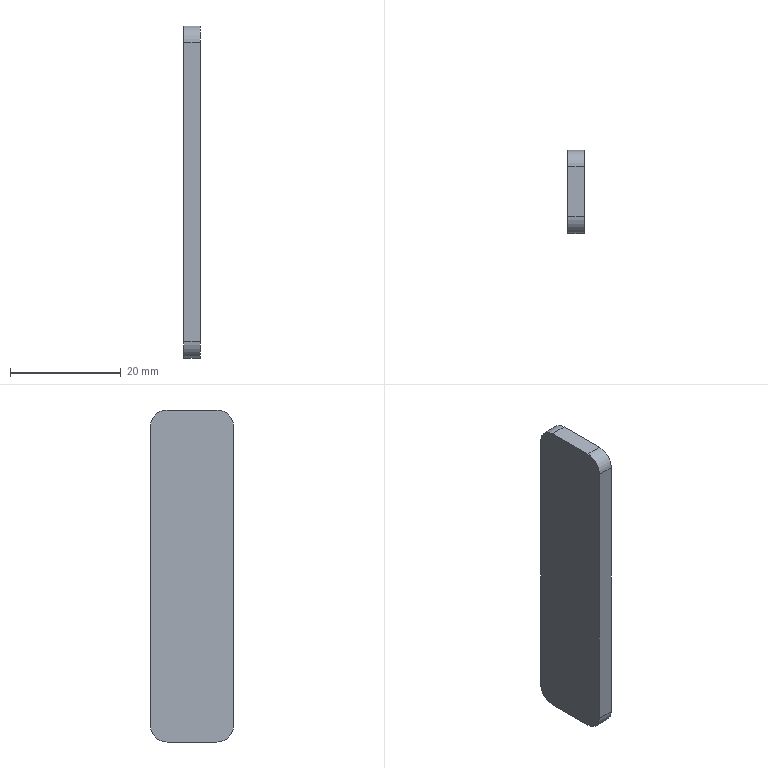Part | SolidWorks | features BaseBody 1 | 1 solid | 10 faces | box 3 x 15 x 60 mm | volume 2677 mm3 | plane 6 | cylinder 4 | commonest cylinder face diameters 6 x4
STEP:
#1=CARTESIAN_POINT('',(72.,-22.5,27.));
#2=VERTEX_POINT('',#1);
#3=CARTESIAN_POINT('',(72.,-25.5,30.));
#4=VERTEX_POINT('',#3);
#5=CARTESIAN_POINT('',(72.,-25.5,27.));
#6=DIRECTION('',(1.,0.,0.));
#7=DIRECTION('',(0.,1.,0.));
#8=AXIS2_PLACEMENT_3D('',#5,#6,#7);
#9=CIRCLE('',#8,3.);
#10=EDGE_CURVE('',#2,#4,#9,.T.);
#11=ORIENTED_EDGE('',*,*,#10,.F.);
#12=CARTESIAN_POINT('',(72.,-22.5,-27.));
#13=VERTEX_POINT('',#12);
#14=CARTESIAN_POINT('',(72.,-22.5,-27.));
#15=DIRECTION('',(0.,0.,1.));
#16=VECTOR('',#15,1000.);
#17=LINE('',#14,#16);
#18=EDGE_CURVE('',#13,#2,#17,.T.);
#19=ORIENTED_EDGE('',*,*,#18,.F.);
#20=CARTESIAN_POINT('',(72.,-25.5,-30.));
#21=VERTEX_POINT('',#20);
#22=CARTESIAN_POINT('',(72.,-25.5,-27.));
#23=DIRECTION('',(1.,0.,0.));
#24=DIRECTION('',(0.,0.,-1.));
#25=AXIS2_PLACEMENT_3D('',#22,#23,#24);
#26=CIRCLE('',#25,3.);
#27=EDGE_CURVE('',#21,#13,#26,.T.);
#28=ORIENTED_EDGE('',*,*,#27,.F.);
#29=CARTESIAN_POINT('',(72.,-34.5,-30.));
#30=VERTEX_POINT('',#29);
#31=CARTESIAN_POINT('',(72.,-34.5,-30.));
#32=DIRECTION('',(0.,1.,0.));
#33=VECTOR('',#32,1000.);
#34=LINE('',#31,#33);
#35=EDGE_CURVE('',#30,#21,#34,.T.);
#36=ORIENTED_EDGE('',*,*,#35,.F.);
#37=CARTESIAN_POINT('',(72.,-37.5,-27.));
#38=VERTEX_POINT('',#37);
#39=CARTESIAN_POINT('',(72.,-34.5,-27.));
#40=DIRECTION('',(1.,0.,0.));
#41=DIRECTION('',(0.,-1.,0.));
#42=AXIS2_PLACEMENT_3D('',#39,#40,#41);
#43=CIRCLE('',#42,3.);
#44=EDGE_CURVE('',#38,#30,#43,.T.);
#45=ORIENTED_EDGE('',*,*,#44,.F.);
#46=CARTESIAN_POINT('',(72.,-37.5,27.));
#47=VERTEX_POINT('',#46);
#48=CARTESIAN_POINT('',(72.,-37.5,27.));
#49=DIRECTION('',(0.,0.,-1.));
#50=VECTOR('',#49,1000.);
#51=LINE('',#48,#50);
#52=EDGE_CURVE('',#47,#38,#51,.T.);
#53=ORIENTED_EDGE('',*,*,#52,.F.);
#54=CARTESIAN_POINT('',(72.,-34.5,30.));
#55=VERTEX_POINT('',#54);
#56=CARTESIAN_POINT('',(72.,-34.5,27.));
#57=DIRECTION('',(1.,0.,0.));
#58=DIRECTION('',(0.,0.,1.));
#59=AXIS2_PLACEMENT_3D('',#56,#57,#58);
#60=CIRCLE('',#59,3.);
#61=EDGE_CURVE('',#55,#47,#60,.T.);
#62=ORIENTED_EDGE('',*,*,#61,.F.);
#63=CARTESIAN_POINT('',(72.,-25.5,30.));
#64=DIRECTION('',(0.,-1.,0.));
#65=VECTOR('',#64,1000.);
#66=LINE('',#63,#65);
#67=EDGE_CURVE('',#4,#55,#66,.T.);
#68=ORIENTED_EDGE('',*,*,#67,.F.);
#69=EDGE_LOOP('',(#11,#19,#28,#36,#45,#53,#62,#68));
#70=FACE_OUTER_BOUND('',#69,.T.);
#71=CARTESIAN_POINT('',(72.,-30.,0.));
#72=DIRECTION('',(-1.,0.,0.));
#73=DIRECTION('',(0.,0.,1.));
#74=AXIS2_PLACEMENT_3D('',#71,#72,#73);
#75=PLANE('',#74);
#76=ADVANCED_FACE('',(#70),#75,.T.);
#77=CARTESIAN_POINT('',(75.,-22.5,27.));
#78=VERTEX_POINT('',#77);
#79=CARTESIAN_POINT('',(75.,-22.5,27.));
#80=DIRECTION('',(-1.,0.,0.));
#81=VECTOR('',#80,1000.);
#82=LINE('',#79,#81);
#83=EDGE_CURVE('',#78,#2,#82,.T.);
#84=ORIENTED_EDGE('',*,*,#83,.F.);
#85=CARTESIAN_POINT('',(75.,-22.5,-27.));
#86=VERTEX_POINT('',#85);
#87=CARTESIAN_POINT('',(75.,-22.5,-27.));
#88=DIRECTION('',(0.,0.,1.));
#89=VECTOR('',#88,1000.);
#90=LINE('',#87,#89);
#91=EDGE_CURVE('',#86,#78,#90,.T.);
#92=ORIENTED_EDGE('',*,*,#91,.F.);
#93=CARTESIAN_POINT('',(72.,-22.5,-27.));
#94=DIRECTION('',(1.,0.,0.));
#95=VECTOR('',#94,1000.);
#96=LINE('',#93,#95);
#97=EDGE_CURVE('',#13,#86,#96,.T.);
#98=ORIENTED_EDGE('',*,*,#97,.F.);
#99=ORIENTED_EDGE('',*,*,#18,.T.);
#100=EDGE_LOOP('',(#84,#92,#98,#99));
#101=FACE_OUTER_BOUND('',#100,.T.);
#102=CARTESIAN_POINT('',(75.,-22.5,30.));
#103=DIRECTION('',(0.,1.,0.));
#104=DIRECTION('',(1.,0.,0.));
#105=AXIS2_PLACEMENT_3D('',#102,#103,#104);
#106=PLANE('',#105);
#107=ADVANCED_FACE('',(#101),#106,.T.);
#108=CARTESIAN_POINT('',(75.,-37.5,27.));
#109=VERTEX_POINT('',#108);
#110=CARTESIAN_POINT('',(72.,-37.5,27.));
#111=DIRECTION('',(1.,0.,0.));
#112=VECTOR('',#111,1000.);
#113=LINE('',#110,#112);
#114=EDGE_CURVE('',#47,#109,#113,.T.);
#115=ORIENTED_EDGE('',*,*,#114,.F.);
#116=ORIENTED_EDGE('',*,*,#52,.T.);
#117=CARTESIAN_POINT('',(75.,-37.5,-27.));
#118=VERTEX_POINT('',#117);
#119=CARTESIAN_POINT('',(75.,-37.5,-27.));
#120=DIRECTION('',(-1.,0.,0.));
#121=VECTOR('',#120,1000.);
#122=LINE('',#119,#121);
#123=EDGE_CURVE('',#118,#38,#122,.T.);
#124=ORIENTED_EDGE('',*,*,#123,.F.);
#125=CARTESIAN_POINT('',(75.,-37.5,27.));
#126=DIRECTION('',(0.,0.,-1.));
#127=VECTOR('',#126,1000.);
#128=LINE('',#125,#127);
#129=EDGE_CURVE('',#109,#118,#128,.T.);
#130=ORIENTED_EDGE('',*,*,#129,.F.);
#131=EDGE_LOOP('',(#115,#116,#124,#130));
#132=FACE_OUTER_BOUND('',#131,.T.);
#133=CARTESIAN_POINT('',(75.,-37.5,-30.));
#134=DIRECTION('',(0.,-1.,0.));
#135=DIRECTION('',(0.,0.,-1.));
#136=AXIS2_PLACEMENT_3D('',#133,#134,#135);
#137=PLANE('',#136);
#138=ADVANCED_FACE('',(#132),#137,.T.);
#139=ORIENTED_EDGE('',*,*,#44,.T.);
#140=CARTESIAN_POINT('',(75.,-34.5,-30.));
#141=VERTEX_POINT('',#140);
#142=CARTESIAN_POINT('',(75.,-34.5,-30.));
#143=DIRECTION('',(-1.,0.,0.));
#144=VECTOR('',#143,1000.);
#145=LINE('',#142,#144);
#146=EDGE_CURVE('',#141,#30,#145,.T.);
#147=ORIENTED_EDGE('',*,*,#146,.F.);
#148=CARTESIAN_POINT('',(75.,-34.5,-27.));
#149=DIRECTION('',(1.,0.,0.));
#150=DIRECTION('',(0.,-1.,0.));
#151=AXIS2_PLACEMENT_3D('',#148,#149,#150);
#152=CIRCLE('',#151,3.);
#153=EDGE_CURVE('',#118,#141,#152,.T.);
#154=ORIENTED_EDGE('',*,*,#153,.F.);
#155=ORIENTED_EDGE('',*,*,#123,.T.);
#156=EDGE_LOOP('',(#139,#147,#154,#155));
#157=FACE_OUTER_BOUND('',#156,.T.);
#158=CARTESIAN_POINT('',(75.,-34.5,-27.));
#159=DIRECTION('',(-1.,0.,0.));
#160=DIRECTION('',(0.,-1.,0.));
#161=AXIS2_PLACEMENT_3D('',#158,#159,#160);
#162=CYLINDRICAL_SURFACE('',#161,3.);
#163=ADVANCED_FACE('',(#157),#162,.T.);
#164=CARTESIAN_POINT('',(75.,-25.5,-30.));
#165=VERTEX_POINT('',#164);
#166=CARTESIAN_POINT('',(75.,-25.5,-30.));
#167=DIRECTION('',(-1.,0.,0.));
#168=VECTOR('',#167,1000.);
#169=LINE('',#166,#168);
#170=EDGE_CURVE('',#165,#21,#169,.T.);
#171=ORIENTED_EDGE('',*,*,#170,.F.);
#172=CARTESIAN_POINT('',(75.,-34.5,-30.));
#173=DIRECTION('',(0.,1.,0.));
#174=VECTOR('',#173,1000.);
#175=LINE('',#172,#174);
#176=EDGE_CURVE('',#141,#165,#175,.T.);
#177=ORIENTED_EDGE('',*,*,#176,.F.);
#178=ORIENTED_EDGE('',*,*,#146,.T.);
#179=ORIENTED_EDGE('',*,*,#35,.T.);
#180=EDGE_LOOP('',(#171,#177,#178,#179));
#181=FACE_OUTER_BOUND('',#180,.T.);
#182=CARTESIAN_POINT('',(75.,-22.5,-30.));
#183=DIRECTION('',(0.,0.,-1.));
#184=DIRECTION('',(0.,-1.,0.));
#185=AXIS2_PLACEMENT_3D('',#182,#183,#184);
#186=PLANE('',#185);
#187=ADVANCED_FACE('',(#181),#186,.T.);
#188=ORIENTED_EDGE('',*,*,#27,.T.);
#189=ORIENTED_EDGE('',*,*,#97,.T.);
#190=CARTESIAN_POINT('',(75.,-25.5,-27.));
#191=DIRECTION('',(1.,0.,0.));
#192=DIRECTION('',(0.,0.,-1.));
#193=AXIS2_PLACEMENT_3D('',#190,#191,#192);
#194=CIRCLE('',#193,3.);
#195=EDGE_CURVE('',#165,#86,#194,.T.);
#196=ORIENTED_EDGE('',*,*,#195,.F.);
#197=ORIENTED_EDGE('',*,*,#170,.T.);
#198=EDGE_LOOP('',(#188,#189,#196,#197));
#199=FACE_OUTER_BOUND('',#198,.T.);
#200=CARTESIAN_POINT('',(75.,-25.5,-27.));
#201=DIRECTION('',(-1.,0.,0.));
#202=DIRECTION('',(0.,0.,-1.));
#203=AXIS2_PLACEMENT_3D('',#200,#201,#202);
#204=CYLINDRICAL_SURFACE('',#203,3.);
#205=ADVANCED_FACE('',(#199),#204,.T.);
#206=ORIENTED_EDGE('',*,*,#61,.T.);
#207=ORIENTED_EDGE('',*,*,#114,.T.);
#208=CARTESIAN_POINT('',(75.,-34.5,30.));
#209=VERTEX_POINT('',#208);
#210=CARTESIAN_POINT('',(75.,-34.5,27.));
#211=DIRECTION('',(1.,0.,0.));
#212=DIRECTION('',(0.,0.,1.));
#213=AXIS2_PLACEMENT_3D('',#210,#211,#212);
#214=CIRCLE('',#213,3.);
#215=EDGE_CURVE('',#209,#109,#214,.T.);
#216=ORIENTED_EDGE('',*,*,#215,.F.);
#217=CARTESIAN_POINT('',(72.,-34.5,30.));
#218=DIRECTION('',(1.,0.,0.));
#219=VECTOR('',#218,1000.);
#220=LINE('',#217,#219);
#221=EDGE_CURVE('',#55,#209,#220,.T.);
#222=ORIENTED_EDGE('',*,*,#221,.F.);
#223=EDGE_LOOP('',(#206,#207,#216,#222));
#224=FACE_OUTER_BOUND('',#223,.T.);
#225=CARTESIAN_POINT('',(75.,-34.5,27.));
#226=DIRECTION('',(-1.,0.,0.));
#227=DIRECTION('',(0.,0.,1.));
#228=AXIS2_PLACEMENT_3D('',#225,#226,#227);
#229=CYLINDRICAL_SURFACE('',#228,3.);
#230=ADVANCED_FACE('',(#224),#229,.T.);
#231=CARTESIAN_POINT('',(75.,-25.5,30.));
#232=VERTEX_POINT('',#231);
#233=CARTESIAN_POINT('',(72.,-25.5,30.));
#234=DIRECTION('',(1.,0.,0.));
#235=VECTOR('',#234,1000.);
#236=LINE('',#233,#235);
#237=EDGE_CURVE('',#4,#232,#236,.T.);
#238=ORIENTED_EDGE('',*,*,#237,.F.);
#239=ORIENTED_EDGE('',*,*,#67,.T.);
#240=ORIENTED_EDGE('',*,*,#221,.T.);
#241=CARTESIAN_POINT('',(75.,-25.5,30.));
#242=DIRECTION('',(0.,-1.,0.));
#243=VECTOR('',#242,1000.);
#244=LINE('',#241,#243);
#245=EDGE_CURVE('',#232,#209,#244,.T.);
#246=ORIENTED_EDGE('',*,*,#245,.F.);
#247=EDGE_LOOP('',(#238,#239,#240,#246));
#248=FACE_OUTER_BOUND('',#247,.T.);
#249=CARTESIAN_POINT('',(75.,-37.5,30.));
#250=DIRECTION('',(0.,0.,1.));
#251=DIRECTION('',(1.,0.,0.));
#252=AXIS2_PLACEMENT_3D('',#249,#250,#251);
#253=PLANE('',#252);
#254=ADVANCED_FACE('',(#248),#253,.T.);
#255=CARTESIAN_POINT('',(75.,-25.5,27.));
#256=DIRECTION('',(-1.,0.,0.));
#257=DIRECTION('',(0.,0.,1.));
#258=AXIS2_PLACEMENT_3D('',#255,#256,#257);
#259=CIRCLE('',#258,3.);
#260=EDGE_CURVE('',#232,#78,#259,.T.);
#261=ORIENTED_EDGE('',*,*,#260,.F.);
#262=ORIENTED_EDGE('',*,*,#245,.T.);
#263=ORIENTED_EDGE('',*,*,#215,.T.);
#264=ORIENTED_EDGE('',*,*,#129,.T.);
#265=ORIENTED_EDGE('',*,*,#153,.T.);
#266=ORIENTED_EDGE('',*,*,#176,.T.);
#267=ORIENTED_EDGE('',*,*,#195,.T.);
#268=ORIENTED_EDGE('',*,*,#91,.T.);
#269=EDGE_LOOP('',(#261,#262,#263,#264,#265,#266,#267,#268));
#270=FACE_OUTER_BOUND('',#269,.T.);
#271=CARTESIAN_POINT('',(75.,-30.,0.));
#272=DIRECTION('',(1.,0.,0.));
#273=DIRECTION('',(0.,1.,0.));
#274=AXIS2_PLACEMENT_3D('',#271,#272,#273);
#275=PLANE('',#274);
#276=ADVANCED_FACE('',(#270),#275,.T.);
#277=ORIENTED_EDGE('',*,*,#10,.T.);
#278=ORIENTED_EDGE('',*,*,#237,.T.);
#279=ORIENTED_EDGE('',*,*,#260,.T.);
#280=ORIENTED_EDGE('',*,*,#83,.T.);
#281=EDGE_LOOP('',(#277,#278,#279,#280));
#282=FACE_OUTER_BOUND('',#281,.T.);
#283=CARTESIAN_POINT('',(75.,-25.5,27.));
#284=DIRECTION('',(-1.,0.,0.));
#285=DIRECTION('',(0.,1.,0.));
#286=AXIS2_PLACEMENT_3D('',#283,#284,#285);
#287=CYLINDRICAL_SURFACE('',#286,3.);
#288=ADVANCED_FACE('',(#282),#287,.T.);
#289=CLOSED_SHELL('',(#76,#107,#138,#163,#187,#205,#230,#254,#276,#288));
#290=MANIFOLD_SOLID_BREP('',#289);
#291=CARTESIAN_POINT('',(0.,0.,0.));
#292=DIRECTION('',(0.,0.,1.));
#293=DIRECTION('',(1.,0.,0.));
#294=AXIS2_PLACEMENT_3D('',#291,#292,#293);
#295=(LENGTH_UNIT()NAMED_UNIT(*)SI_UNIT(.MILLI.,.METRE.));
#296=UNCERTAINTY_MEASURE_WITH_UNIT(LENGTH_MEASURE(0.00001),#295,'','');
#297=(NAMED_UNIT(*)PLANE_ANGLE_UNIT()SI_UNIT($,.RADIAN.));
#298=(NAMED_UNIT(*)SI_UNIT($,.STERADIAN.)SOLID_ANGLE_UNIT());
#299=(GEOMETRIC_REPRESENTATION_CONTEXT(3)GLOBAL_UNCERTAINTY_ASSIGNED_CONTEXT((#296))GLOBAL_UNIT_ASSIGNED_CONTEXT((#295,#297,#298))REPRESENTATION_CONTEXT('',''));
#300=ADVANCED_BREP_SHAPE_REPRESENTATION('',(#290,#294),#299);